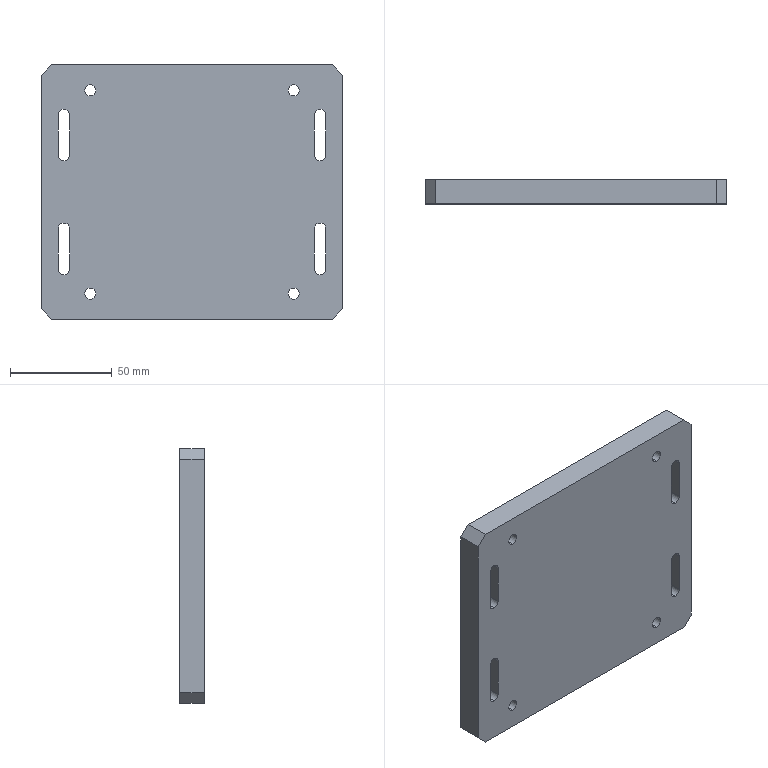Part | STEP file | ND25021-01-JDKM-68-TL | 1 solid | 50 faces | box 148 x 12 x 125 mm | volume 212656 mm3 | cylinder 28 | plane 22 | commonest cylinder face diameters 5.5 x20 10 x8